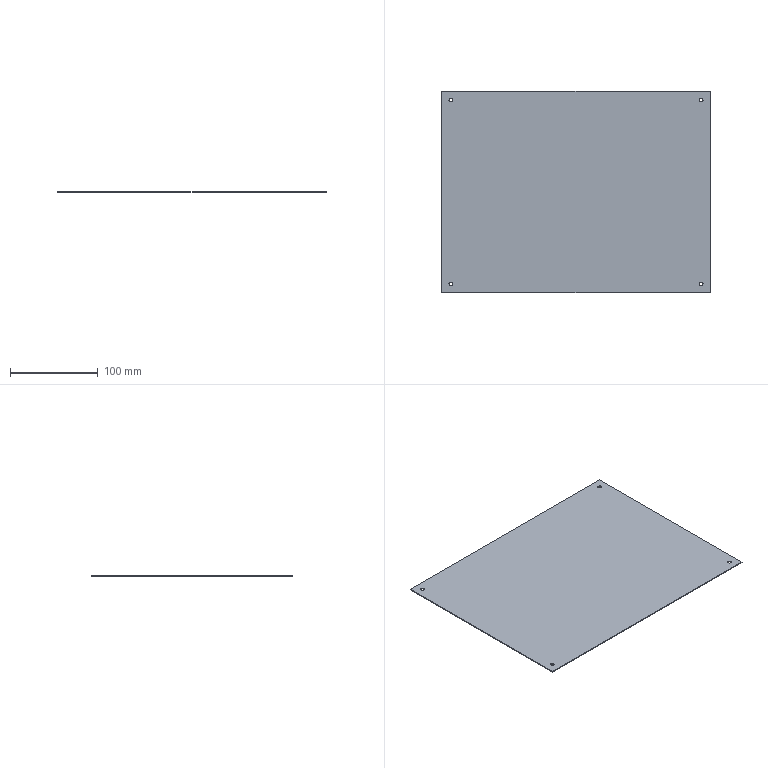Part | SolidWorks | features BaseBody 1 | 1 solid | 14 faces | box 306 x 230 x 1 mm | volume 70330 mm3 | cylinder 8 | plane 6 | commonest cylinder face diameters 4 x8
STEP:
#1=CARTESIAN_POINT('',(-141.,105.,1.));
#2=VERTEX_POINT('',#1);
#3=CARTESIAN_POINT('',(-141.,105.,0.));
#4=VERTEX_POINT('',#3);
#5=CARTESIAN_POINT('',(-141.,105.,1.));
#6=DIRECTION('',(0.,0.,-1.));
#7=VECTOR('',#6,1000.);
#8=LINE('',#5,#7);
#9=EDGE_CURVE('',#2,#4,#8,.T.);
#10=ORIENTED_EDGE('',*,*,#9,.F.);
#11=CARTESIAN_POINT('',(-145.,105.,1.));
#12=VERTEX_POINT('',#11);
#13=CARTESIAN_POINT('',(-143.,105.,1.));
#14=DIRECTION('',(0.,0.,-1.));
#15=DIRECTION('',(-1.,0.,0.));
#16=AXIS2_PLACEMENT_3D('',#13,#14,#15);
#17=CIRCLE('',#16,2.);
#18=EDGE_CURVE('',#12,#2,#17,.T.);
#19=ORIENTED_EDGE('',*,*,#18,.F.);
#20=CARTESIAN_POINT('',(-145.,105.,0.));
#21=VERTEX_POINT('',#20);
#22=CARTESIAN_POINT('',(-145.,105.,1.));
#23=DIRECTION('',(0.,0.,-1.));
#24=VECTOR('',#23,1000.);
#25=LINE('',#22,#24);
#26=EDGE_CURVE('',#12,#21,#25,.T.);
#27=ORIENTED_EDGE('',*,*,#26,.T.);
#28=CARTESIAN_POINT('',(-143.,105.,0.));
#29=DIRECTION('',(0.,0.,-1.));
#30=DIRECTION('',(-1.,0.,0.));
#31=AXIS2_PLACEMENT_3D('',#28,#29,#30);
#32=CIRCLE('',#31,2.);
#33=EDGE_CURVE('',#21,#4,#32,.T.);
#34=ORIENTED_EDGE('',*,*,#33,.T.);
#35=EDGE_LOOP('',(#10,#19,#27,#34));
#36=FACE_OUTER_BOUND('',#35,.T.);
#37=CARTESIAN_POINT('',(-143.,105.,1.));
#38=DIRECTION('',(0.,0.,-1.));
#39=DIRECTION('',(-1.,0.,0.));
#40=AXIS2_PLACEMENT_3D('',#37,#38,#39);
#41=CYLINDRICAL_SURFACE('',#40,2.);
#42=ADVANCED_FACE('',(#36),#41,.F.);
#43=CARTESIAN_POINT('',(-141.,-105.,1.));
#44=VERTEX_POINT('',#43);
#45=CARTESIAN_POINT('',(-141.,-105.,0.));
#46=VERTEX_POINT('',#45);
#47=CARTESIAN_POINT('',(-141.,-105.,1.));
#48=DIRECTION('',(0.,0.,-1.));
#49=VECTOR('',#48,1000.);
#50=LINE('',#47,#49);
#51=EDGE_CURVE('',#44,#46,#50,.T.);
#52=ORIENTED_EDGE('',*,*,#51,.F.);
#53=CARTESIAN_POINT('',(-145.,-105.,1.));
#54=VERTEX_POINT('',#53);
#55=CARTESIAN_POINT('',(-143.,-105.,1.));
#56=DIRECTION('',(0.,0.,-1.));
#57=DIRECTION('',(-1.,0.,0.));
#58=AXIS2_PLACEMENT_3D('',#55,#56,#57);
#59=CIRCLE('',#58,2.);
#60=EDGE_CURVE('',#54,#44,#59,.T.);
#61=ORIENTED_EDGE('',*,*,#60,.F.);
#62=CARTESIAN_POINT('',(-145.,-105.,0.));
#63=VERTEX_POINT('',#62);
#64=CARTESIAN_POINT('',(-145.,-105.,1.));
#65=DIRECTION('',(0.,0.,-1.));
#66=VECTOR('',#65,1000.);
#67=LINE('',#64,#66);
#68=EDGE_CURVE('',#54,#63,#67,.T.);
#69=ORIENTED_EDGE('',*,*,#68,.T.);
#70=CARTESIAN_POINT('',(-143.,-105.,0.));
#71=DIRECTION('',(0.,0.,-1.));
#72=DIRECTION('',(-1.,0.,0.));
#73=AXIS2_PLACEMENT_3D('',#70,#71,#72);
#74=CIRCLE('',#73,2.);
#75=EDGE_CURVE('',#63,#46,#74,.T.);
#76=ORIENTED_EDGE('',*,*,#75,.T.);
#77=EDGE_LOOP('',(#52,#61,#69,#76));
#78=FACE_OUTER_BOUND('',#77,.T.);
#79=CARTESIAN_POINT('',(-143.,-105.,1.));
#80=DIRECTION('',(0.,0.,-1.));
#81=DIRECTION('',(-1.,0.,0.));
#82=AXIS2_PLACEMENT_3D('',#79,#80,#81);
#83=CYLINDRICAL_SURFACE('',#82,2.);
#84=ADVANCED_FACE('',(#78),#83,.F.);
#85=CARTESIAN_POINT('',(145.,-105.,1.));
#86=VERTEX_POINT('',#85);
#87=CARTESIAN_POINT('',(145.,-105.,0.));
#88=VERTEX_POINT('',#87);
#89=CARTESIAN_POINT('',(145.,-105.,1.));
#90=DIRECTION('',(0.,0.,-1.));
#91=VECTOR('',#90,1000.);
#92=LINE('',#89,#91);
#93=EDGE_CURVE('',#86,#88,#92,.T.);
#94=ORIENTED_EDGE('',*,*,#93,.F.);
#95=CARTESIAN_POINT('',(141.,-105.,1.));
#96=VERTEX_POINT('',#95);
#97=CARTESIAN_POINT('',(143.,-105.,1.));
#98=DIRECTION('',(0.,0.,-1.));
#99=DIRECTION('',(-1.,0.,0.));
#100=AXIS2_PLACEMENT_3D('',#97,#98,#99);
#101=CIRCLE('',#100,2.);
#102=EDGE_CURVE('',#96,#86,#101,.T.);
#103=ORIENTED_EDGE('',*,*,#102,.F.);
#104=CARTESIAN_POINT('',(141.,-105.,0.));
#105=VERTEX_POINT('',#104);
#106=CARTESIAN_POINT('',(141.,-105.,1.));
#107=DIRECTION('',(0.,0.,-1.));
#108=VECTOR('',#107,1000.);
#109=LINE('',#106,#108);
#110=EDGE_CURVE('',#96,#105,#109,.T.);
#111=ORIENTED_EDGE('',*,*,#110,.T.);
#112=CARTESIAN_POINT('',(143.,-105.,0.));
#113=DIRECTION('',(0.,0.,-1.));
#114=DIRECTION('',(-1.,0.,0.));
#115=AXIS2_PLACEMENT_3D('',#112,#113,#114);
#116=CIRCLE('',#115,2.);
#117=EDGE_CURVE('',#105,#88,#116,.T.);
#118=ORIENTED_EDGE('',*,*,#117,.T.);
#119=EDGE_LOOP('',(#94,#103,#111,#118));
#120=FACE_OUTER_BOUND('',#119,.T.);
#121=CARTESIAN_POINT('',(143.,-105.,1.));
#122=DIRECTION('',(0.,0.,-1.));
#123=DIRECTION('',(-1.,0.,0.));
#124=AXIS2_PLACEMENT_3D('',#121,#122,#123);
#125=CYLINDRICAL_SURFACE('',#124,2.);
#126=ADVANCED_FACE('',(#120),#125,.F.);
#127=CARTESIAN_POINT('',(145.,105.,1.));
#128=VERTEX_POINT('',#127);
#129=CARTESIAN_POINT('',(145.,105.,0.));
#130=VERTEX_POINT('',#129);
#131=CARTESIAN_POINT('',(145.,105.,1.));
#132=DIRECTION('',(0.,0.,-1.));
#133=VECTOR('',#132,1000.);
#134=LINE('',#131,#133);
#135=EDGE_CURVE('',#128,#130,#134,.T.);
#136=ORIENTED_EDGE('',*,*,#135,.F.);
#137=CARTESIAN_POINT('',(141.,105.,1.));
#138=VERTEX_POINT('',#137);
#139=CARTESIAN_POINT('',(143.,105.,1.));
#140=DIRECTION('',(0.,0.,-1.));
#141=DIRECTION('',(-1.,0.,0.));
#142=AXIS2_PLACEMENT_3D('',#139,#140,#141);
#143=CIRCLE('',#142,2.);
#144=EDGE_CURVE('',#138,#128,#143,.T.);
#145=ORIENTED_EDGE('',*,*,#144,.F.);
#146=CARTESIAN_POINT('',(141.,105.,0.));
#147=VERTEX_POINT('',#146);
#148=CARTESIAN_POINT('',(141.,105.,1.));
#149=DIRECTION('',(0.,0.,-1.));
#150=VECTOR('',#149,1000.);
#151=LINE('',#148,#150);
#152=EDGE_CURVE('',#138,#147,#151,.T.);
#153=ORIENTED_EDGE('',*,*,#152,.T.);
#154=CARTESIAN_POINT('',(143.,105.,0.));
#155=DIRECTION('',(0.,0.,-1.));
#156=DIRECTION('',(-1.,0.,0.));
#157=AXIS2_PLACEMENT_3D('',#154,#155,#156);
#158=CIRCLE('',#157,2.);
#159=EDGE_CURVE('',#147,#130,#158,.T.);
#160=ORIENTED_EDGE('',*,*,#159,.T.);
#161=EDGE_LOOP('',(#136,#145,#153,#160));
#162=FACE_OUTER_BOUND('',#161,.T.);
#163=CARTESIAN_POINT('',(143.,105.,1.));
#164=DIRECTION('',(0.,0.,-1.));
#165=DIRECTION('',(-1.,0.,0.));
#166=AXIS2_PLACEMENT_3D('',#163,#164,#165);
#167=CYLINDRICAL_SURFACE('',#166,2.);
#168=ADVANCED_FACE('',(#162),#167,.F.);
#169=ORIENTED_EDGE('',*,*,#159,.F.);
#170=CARTESIAN_POINT('',(143.,105.,0.));
#171=DIRECTION('',(0.,0.,-1.));
#172=DIRECTION('',(-1.,0.,0.));
#173=AXIS2_PLACEMENT_3D('',#170,#171,#172);
#174=CIRCLE('',#173,2.);
#175=EDGE_CURVE('',#130,#147,#174,.T.);
#176=ORIENTED_EDGE('',*,*,#175,.F.);
#177=EDGE_LOOP('',(#169,#176));
#178=FACE_BOUND('',#177,.T.);
#179=ORIENTED_EDGE('',*,*,#117,.F.);
#180=CARTESIAN_POINT('',(143.,-105.,0.));
#181=DIRECTION('',(0.,0.,-1.));
#182=DIRECTION('',(-1.,0.,0.));
#183=AXIS2_PLACEMENT_3D('',#180,#181,#182);
#184=CIRCLE('',#183,2.);
#185=EDGE_CURVE('',#88,#105,#184,.T.);
#186=ORIENTED_EDGE('',*,*,#185,.F.);
#187=EDGE_LOOP('',(#179,#186));
#188=FACE_BOUND('',#187,.T.);
#189=ORIENTED_EDGE('',*,*,#75,.F.);
#190=CARTESIAN_POINT('',(-143.,-105.,0.));
#191=DIRECTION('',(0.,0.,-1.));
#192=DIRECTION('',(-1.,0.,0.));
#193=AXIS2_PLACEMENT_3D('',#190,#191,#192);
#194=CIRCLE('',#193,2.);
#195=EDGE_CURVE('',#46,#63,#194,.T.);
#196=ORIENTED_EDGE('',*,*,#195,.F.);
#197=EDGE_LOOP('',(#189,#196));
#198=FACE_BOUND('',#197,.T.);
#199=ORIENTED_EDGE('',*,*,#33,.F.);
#200=CARTESIAN_POINT('',(-143.,105.,0.));
#201=DIRECTION('',(0.,0.,-1.));
#202=DIRECTION('',(-1.,0.,0.));
#203=AXIS2_PLACEMENT_3D('',#200,#201,#202);
#204=CIRCLE('',#203,2.);
#205=EDGE_CURVE('',#4,#21,#204,.T.);
#206=ORIENTED_EDGE('',*,*,#205,.F.);
#207=EDGE_LOOP('',(#199,#206));
#208=FACE_BOUND('',#207,.T.);
#209=CARTESIAN_POINT('',(-153.,115.,0.));
#210=VERTEX_POINT('',#209);
#211=CARTESIAN_POINT('',(-153.,-115.,0.));
#212=VERTEX_POINT('',#211);
#213=CARTESIAN_POINT('',(-153.,115.,0.));
#214=DIRECTION('',(0.,-1.,0.));
#215=VECTOR('',#214,1000.);
#216=LINE('',#213,#215);
#217=EDGE_CURVE('',#210,#212,#216,.T.);
#218=ORIENTED_EDGE('',*,*,#217,.F.);
#219=CARTESIAN_POINT('',(153.,115.,0.));
#220=VERTEX_POINT('',#219);
#221=CARTESIAN_POINT('',(153.,115.,0.));
#222=DIRECTION('',(-1.,0.,0.));
#223=VECTOR('',#222,1000.);
#224=LINE('',#221,#223);
#225=EDGE_CURVE('',#220,#210,#224,.T.);
#226=ORIENTED_EDGE('',*,*,#225,.F.);
#227=CARTESIAN_POINT('',(153.,-115.,0.));
#228=VERTEX_POINT('',#227);
#229=CARTESIAN_POINT('',(153.,115.,0.));
#230=DIRECTION('',(0.,1.,0.));
#231=VECTOR('',#230,1000.);
#232=LINE('',#229,#231);
#233=EDGE_CURVE('',#228,#220,#232,.T.);
#234=ORIENTED_EDGE('',*,*,#233,.F.);
#235=CARTESIAN_POINT('',(153.,-115.,0.));
#236=DIRECTION('',(1.,0.,0.));
#237=VECTOR('',#236,1000.);
#238=LINE('',#235,#237);
#239=EDGE_CURVE('',#212,#228,#238,.T.);
#240=ORIENTED_EDGE('',*,*,#239,.F.);
#241=EDGE_LOOP('',(#218,#226,#234,#240));
#242=FACE_OUTER_BOUND('',#241,.T.);
#243=CARTESIAN_POINT('',(0.,0.,0.));
#244=DIRECTION('',(0.,0.,-1.));
#245=DIRECTION('',(0.,-1.,0.));
#246=AXIS2_PLACEMENT_3D('',#243,#244,#245);
#247=PLANE('',#246);
#248=ADVANCED_FACE('',(#178,#188,#198,#208,#242),#247,.T.);
#249=ORIENTED_EDGE('',*,*,#144,.T.);
#250=CARTESIAN_POINT('',(143.,105.,1.));
#251=DIRECTION('',(0.,0.,-1.));
#252=DIRECTION('',(-1.,0.,0.));
#253=AXIS2_PLACEMENT_3D('',#250,#251,#252);
#254=CIRCLE('',#253,2.);
#255=EDGE_CURVE('',#128,#138,#254,.T.);
#256=ORIENTED_EDGE('',*,*,#255,.T.);
#257=EDGE_LOOP('',(#249,#256));
#258=FACE_BOUND('',#257,.T.);
#259=ORIENTED_EDGE('',*,*,#102,.T.);
#260=CARTESIAN_POINT('',(143.,-105.,1.));
#261=DIRECTION('',(0.,0.,-1.));
#262=DIRECTION('',(-1.,0.,0.));
#263=AXIS2_PLACEMENT_3D('',#260,#261,#262);
#264=CIRCLE('',#263,2.);
#265=EDGE_CURVE('',#86,#96,#264,.T.);
#266=ORIENTED_EDGE('',*,*,#265,.T.);
#267=EDGE_LOOP('',(#259,#266));
#268=FACE_BOUND('',#267,.T.);
#269=ORIENTED_EDGE('',*,*,#60,.T.);
#270=CARTESIAN_POINT('',(-143.,-105.,1.));
#271=DIRECTION('',(0.,0.,-1.));
#272=DIRECTION('',(-1.,0.,0.));
#273=AXIS2_PLACEMENT_3D('',#270,#271,#272);
#274=CIRCLE('',#273,2.);
#275=EDGE_CURVE('',#44,#54,#274,.T.);
#276=ORIENTED_EDGE('',*,*,#275,.T.);
#277=EDGE_LOOP('',(#269,#276));
#278=FACE_BOUND('',#277,.T.);
#279=ORIENTED_EDGE('',*,*,#18,.T.);
#280=CARTESIAN_POINT('',(-143.,105.,1.));
#281=DIRECTION('',(0.,0.,-1.));
#282=DIRECTION('',(-1.,0.,0.));
#283=AXIS2_PLACEMENT_3D('',#280,#281,#282);
#284=CIRCLE('',#283,2.);
#285=EDGE_CURVE('',#2,#12,#284,.T.);
#286=ORIENTED_EDGE('',*,*,#285,.T.);
#287=EDGE_LOOP('',(#279,#286));
#288=FACE_BOUND('',#287,.T.);
#289=CARTESIAN_POINT('',(-153.,115.,1.));
#290=VERTEX_POINT('',#289);
#291=CARTESIAN_POINT('',(-153.,-115.,1.));
#292=VERTEX_POINT('',#291);
#293=CARTESIAN_POINT('',(-153.,115.,1.));
#294=DIRECTION('',(0.,-1.,0.));
#295=VECTOR('',#294,1000.);
#296=LINE('',#293,#295);
#297=EDGE_CURVE('',#290,#292,#296,.T.);
#298=ORIENTED_EDGE('',*,*,#297,.T.);
#299=CARTESIAN_POINT('',(153.,-115.,1.));
#300=VERTEX_POINT('',#299);
#301=CARTESIAN_POINT('',(153.,-115.,1.));
#302=DIRECTION('',(1.,0.,0.));
#303=VECTOR('',#302,1000.);
#304=LINE('',#301,#303);
#305=EDGE_CURVE('',#292,#300,#304,.T.);
#306=ORIENTED_EDGE('',*,*,#305,.T.);
#307=CARTESIAN_POINT('',(153.,115.,1.));
#308=VERTEX_POINT('',#307);
#309=CARTESIAN_POINT('',(153.,115.,1.));
#310=DIRECTION('',(0.,1.,0.));
#311=VECTOR('',#310,1000.);
#312=LINE('',#309,#311);
#313=EDGE_CURVE('',#300,#308,#312,.T.);
#314=ORIENTED_EDGE('',*,*,#313,.T.);
#315=CARTESIAN_POINT('',(153.,115.,1.));
#316=DIRECTION('',(-1.,0.,0.));
#317=VECTOR('',#316,1000.);
#318=LINE('',#315,#317);
#319=EDGE_CURVE('',#308,#290,#318,.T.);
#320=ORIENTED_EDGE('',*,*,#319,.T.);
#321=EDGE_LOOP('',(#298,#306,#314,#320));
#322=FACE_OUTER_BOUND('',#321,.T.);
#323=CARTESIAN_POINT('',(0.,0.,1.));
#324=DIRECTION('',(0.,0.,-1.));
#325=DIRECTION('',(0.,-1.,0.));
#326=AXIS2_PLACEMENT_3D('',#323,#324,#325);
#327=PLANE('',#326);
#328=ADVANCED_FACE('',(#258,#268,#278,#288,#322),#327,.F.);
#329=ORIENTED_EDGE('',*,*,#225,.T.);
#330=CARTESIAN_POINT('',(-153.,115.,1.));
#331=DIRECTION('',(0.,0.,-1.));
#332=VECTOR('',#331,1000.);
#333=LINE('',#330,#332);
#334=EDGE_CURVE('',#290,#210,#333,.T.);
#335=ORIENTED_EDGE('',*,*,#334,.F.);
#336=ORIENTED_EDGE('',*,*,#319,.F.);
#337=CARTESIAN_POINT('',(153.,115.,1.));
#338=DIRECTION('',(0.,0.,-1.));
#339=VECTOR('',#338,1000.);
#340=LINE('',#337,#339);
#341=EDGE_CURVE('',#308,#220,#340,.T.);
#342=ORIENTED_EDGE('',*,*,#341,.T.);
#343=EDGE_LOOP('',(#329,#335,#336,#342));
#344=FACE_OUTER_BOUND('',#343,.T.);
#345=CARTESIAN_POINT('',(153.,115.,1.));
#346=DIRECTION('',(0.,-1.,0.));
#347=DIRECTION('',(0.,0.,-1.));
#348=AXIS2_PLACEMENT_3D('',#345,#346,#347);
#349=PLANE('',#348);
#350=ADVANCED_FACE('',(#344),#349,.F.);
#351=ORIENTED_EDGE('',*,*,#233,.T.);
#352=ORIENTED_EDGE('',*,*,#341,.F.);
#353=ORIENTED_EDGE('',*,*,#313,.F.);
#354=CARTESIAN_POINT('',(153.,-115.,1.));
#355=DIRECTION('',(0.,0.,-1.));
#356=VECTOR('',#355,1000.);
#357=LINE('',#354,#356);
#358=EDGE_CURVE('',#300,#228,#357,.T.);
#359=ORIENTED_EDGE('',*,*,#358,.T.);
#360=EDGE_LOOP('',(#351,#352,#353,#359));
#361=FACE_OUTER_BOUND('',#360,.T.);
#362=CARTESIAN_POINT('',(153.,115.,1.));
#363=DIRECTION('',(-1.,0.,0.));
#364=DIRECTION('',(0.,0.,1.));
#365=AXIS2_PLACEMENT_3D('',#362,#363,#364);
#366=PLANE('',#365);
#367=ADVANCED_FACE('',(#361),#366,.F.);
#368=ORIENTED_EDGE('',*,*,#239,.T.);
#369=ORIENTED_EDGE('',*,*,#358,.F.);
#370=ORIENTED_EDGE('',*,*,#305,.F.);
#371=CARTESIAN_POINT('',(-153.,-115.,1.));
#372=DIRECTION('',(0.,0.,-1.));
#373=VECTOR('',#372,1000.);
#374=LINE('',#371,#373);
#375=EDGE_CURVE('',#292,#212,#374,.T.);
#376=ORIENTED_EDGE('',*,*,#375,.T.);
#377=EDGE_LOOP('',(#368,#369,#370,#376));
#378=FACE_OUTER_BOUND('',#377,.T.);
#379=CARTESIAN_POINT('',(153.,-115.,1.));
#380=DIRECTION('',(0.,1.,0.));
#381=DIRECTION('',(1.,0.,0.));
#382=AXIS2_PLACEMENT_3D('',#379,#380,#381);
#383=PLANE('',#382);
#384=ADVANCED_FACE('',(#378),#383,.F.);
#385=ORIENTED_EDGE('',*,*,#217,.T.);
#386=ORIENTED_EDGE('',*,*,#375,.F.);
#387=ORIENTED_EDGE('',*,*,#297,.F.);
#388=ORIENTED_EDGE('',*,*,#334,.T.);
#389=EDGE_LOOP('',(#385,#386,#387,#388));
#390=FACE_OUTER_BOUND('',#389,.T.);
#391=CARTESIAN_POINT('',(-153.,115.,1.));
#392=DIRECTION('',(1.,0.,0.));
#393=DIRECTION('',(0.,1.,0.));
#394=AXIS2_PLACEMENT_3D('',#391,#392,#393);
#395=PLANE('',#394);
#396=ADVANCED_FACE('',(#390),#395,.F.);
#397=ORIENTED_EDGE('',*,*,#255,.F.);
#398=ORIENTED_EDGE('',*,*,#135,.T.);
#399=ORIENTED_EDGE('',*,*,#175,.T.);
#400=ORIENTED_EDGE('',*,*,#152,.F.);
#401=EDGE_LOOP('',(#397,#398,#399,#400));
#402=FACE_OUTER_BOUND('',#401,.T.);
#403=CARTESIAN_POINT('',(143.,105.,1.));
#404=DIRECTION('',(0.,0.,-1.));
#405=DIRECTION('',(-1.,0.,0.));
#406=AXIS2_PLACEMENT_3D('',#403,#404,#405);
#407=CYLINDRICAL_SURFACE('',#406,2.);
#408=ADVANCED_FACE('',(#402),#407,.F.);
#409=ORIENTED_EDGE('',*,*,#265,.F.);
#410=ORIENTED_EDGE('',*,*,#93,.T.);
#411=ORIENTED_EDGE('',*,*,#185,.T.);
#412=ORIENTED_EDGE('',*,*,#110,.F.);
#413=EDGE_LOOP('',(#409,#410,#411,#412));
#414=FACE_OUTER_BOUND('',#413,.T.);
#415=CARTESIAN_POINT('',(143.,-105.,1.));
#416=DIRECTION('',(0.,0.,-1.));
#417=DIRECTION('',(-1.,0.,0.));
#418=AXIS2_PLACEMENT_3D('',#415,#416,#417);
#419=CYLINDRICAL_SURFACE('',#418,2.);
#420=ADVANCED_FACE('',(#414),#419,.F.);
#421=ORIENTED_EDGE('',*,*,#275,.F.);
#422=ORIENTED_EDGE('',*,*,#51,.T.);
#423=ORIENTED_EDGE('',*,*,#195,.T.);
#424=ORIENTED_EDGE('',*,*,#68,.F.);
#425=EDGE_LOOP('',(#421,#422,#423,#424));
#426=FACE_OUTER_BOUND('',#425,.T.);
#427=CARTESIAN_POINT('',(-143.,-105.,1.));
#428=DIRECTION('',(0.,0.,-1.));
#429=DIRECTION('',(-1.,0.,0.));
#430=AXIS2_PLACEMENT_3D('',#427,#428,#429);
#431=CYLINDRICAL_SURFACE('',#430,2.);
#432=ADVANCED_FACE('',(#426),#431,.F.);
#433=ORIENTED_EDGE('',*,*,#285,.F.);
#434=ORIENTED_EDGE('',*,*,#9,.T.);
#435=ORIENTED_EDGE('',*,*,#205,.T.);
#436=ORIENTED_EDGE('',*,*,#26,.F.);
#437=EDGE_LOOP('',(#433,#434,#435,#436));
#438=FACE_OUTER_BOUND('',#437,.T.);
#439=CARTESIAN_POINT('',(-143.,105.,1.));
#440=DIRECTION('',(0.,0.,-1.));
#441=DIRECTION('',(-1.,0.,0.));
#442=AXIS2_PLACEMENT_3D('',#439,#440,#441);
#443=CYLINDRICAL_SURFACE('',#442,2.);
#444=ADVANCED_FACE('',(#438),#443,.F.);
#445=CLOSED_SHELL('',(#42,#84,#126,#168,#248,#328,#350,#367,#384,#396,#408,#420,#432,#444));
#446=MANIFOLD_SOLID_BREP('',#445);
#447=CARTESIAN_POINT('',(0.,0.,0.));
#448=DIRECTION('',(0.,0.,1.));
#449=DIRECTION('',(1.,0.,0.));
#450=AXIS2_PLACEMENT_3D('',#447,#448,#449);
#451=(LENGTH_UNIT()NAMED_UNIT(*)SI_UNIT(.MILLI.,.METRE.));
#452=UNCERTAINTY_MEASURE_WITH_UNIT(LENGTH_MEASURE(0.00001),#451,'','');
#453=(NAMED_UNIT(*)PLANE_ANGLE_UNIT()SI_UNIT($,.RADIAN.));
#454=(NAMED_UNIT(*)SI_UNIT($,.STERADIAN.)SOLID_ANGLE_UNIT());
#455=(GEOMETRIC_REPRESENTATION_CONTEXT(3)GLOBAL_UNCERTAINTY_ASSIGNED_CONTEXT((#452))GLOBAL_UNIT_ASSIGNED_CONTEXT((#451,#453,#454))REPRESENTATION_CONTEXT('',''));
#456=ADVANCED_BREP_SHAPE_REPRESENTATION('',(#446,#450),#455);